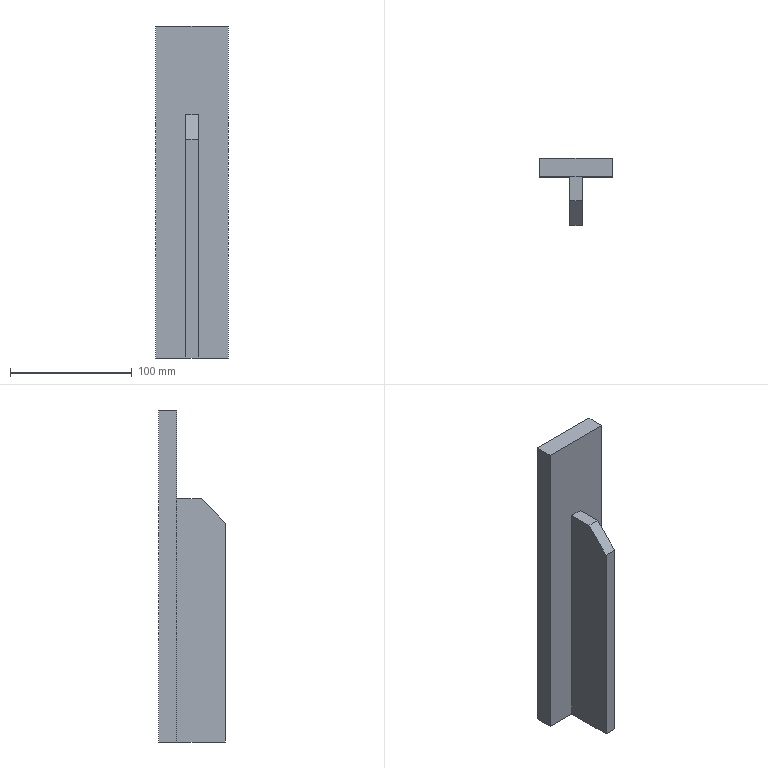Part | NX | features solid 2 | 1 solid | 11 faces | box 60 x 55 x 272.979 mm | volume 323681 mm3 | plane 11
STEP:
#1=CARTESIAN_POINT('',(5.,847.5,-310.));
#2=VERTEX_POINT('',#1);
#3=CARTESIAN_POINT('',(65.,847.5,-310.));
#4=VERTEX_POINT('',#3);
#5=CARTESIAN_POINT('',(9.058,847.5,-310.));
#6=DIRECTION('',(-1.,0.,0.));
#7=VECTOR('',#6,1000.);
#8=LINE('',#5,#7);
#9=EDGE_CURVE('',#2,#4,#8,.F.);
#10=ORIENTED_EDGE('',*,*,#9,.T.);
#11=CARTESIAN_POINT('',(65.,832.5,-310.));
#12=VERTEX_POINT('',#11);
#13=CARTESIAN_POINT('',(65.,840.,-310.));
#14=DIRECTION('',(0.,-1.,0.));
#15=VECTOR('',#14,1000.);
#16=LINE('',#13,#15);
#17=EDGE_CURVE('',#12,#4,#16,.F.);
#18=ORIENTED_EDGE('',*,*,#17,.F.);
#19=CARTESIAN_POINT('',(40.,832.5,-310.));
#20=VERTEX_POINT('',#19);
#21=CARTESIAN_POINT('',(9.058,832.5,-310.));
#22=DIRECTION('',(-1.,0.,0.));
#23=VECTOR('',#22,1000.);
#24=LINE('',#21,#23);
#25=EDGE_CURVE('',#20,#12,#24,.F.);
#26=ORIENTED_EDGE('',*,*,#25,.F.);
#27=CARTESIAN_POINT('',(40.,792.5,-310.));
#28=VERTEX_POINT('',#27);
#29=CARTESIAN_POINT('',(40.,832.5,-310.));
#30=DIRECTION('',(0.,-1.,0.));
#31=VECTOR('',#30,1000.);
#32=LINE('',#29,#31);
#33=EDGE_CURVE('',#20,#28,#32,.T.);
#34=ORIENTED_EDGE('',*,*,#33,.T.);
#35=CARTESIAN_POINT('',(30.,792.5,-310.));
#36=VERTEX_POINT('',#35);
#37=CARTESIAN_POINT('',(35.,792.5,-310.));
#38=DIRECTION('',(1.,0.,0.));
#39=VECTOR('',#38,1000.);
#40=LINE('',#37,#39);
#41=EDGE_CURVE('',#36,#28,#40,.T.);
#42=ORIENTED_EDGE('',*,*,#41,.F.);
#43=CARTESIAN_POINT('',(30.,832.5,-310.));
#44=VERTEX_POINT('',#43);
#45=CARTESIAN_POINT('',(30.,832.5,-310.));
#46=DIRECTION('',(0.,-1.,0.));
#47=VECTOR('',#46,1000.);
#48=LINE('',#45,#47);
#49=EDGE_CURVE('',#44,#36,#48,.T.);
#50=ORIENTED_EDGE('',*,*,#49,.F.);
#51=CARTESIAN_POINT('',(5.,832.5,-310.));
#52=VERTEX_POINT('',#51);
#53=CARTESIAN_POINT('',(9.058,832.5,-310.));
#54=DIRECTION('',(-1.,0.,0.));
#55=VECTOR('',#54,1000.);
#56=LINE('',#53,#55);
#57=EDGE_CURVE('',#52,#44,#56,.F.);
#58=ORIENTED_EDGE('',*,*,#57,.F.);
#59=CARTESIAN_POINT('',(5.,840.,-310.));
#60=DIRECTION('',(0.,-1.,0.));
#61=VECTOR('',#60,1000.);
#62=LINE('',#59,#61);
#63=EDGE_CURVE('',#52,#2,#62,.F.);
#64=ORIENTED_EDGE('',*,*,#63,.T.);
#65=EDGE_LOOP('',(#10,#18,#26,#34,#42,#50,#58,#64));
#66=FACE_BOUND('',#65,.T.);
#67=CARTESIAN_POINT('',(5.,847.5,-310.));
#68=DIRECTION('',(0.,0.,-1.));
#69=DIRECTION('',(-1.,0.,0.));
#70=AXIS2_PLACEMENT_3D('',#67,#68,#69);
#71=PLANE('',#70);
#72=ADVANCED_FACE('',(#66),#71,.T.);
#73=CARTESIAN_POINT('',(30.,812.5,-110.));
#74=VERTEX_POINT('',#73);
#75=CARTESIAN_POINT('',(30.,792.5,-130.));
#76=VERTEX_POINT('',#75);
#77=CARTESIAN_POINT('',(30.,792.5,-130.));
#78=DIRECTION('',(0.,-0.7071,-0.7071));
#79=VECTOR('',#78,1000.);
#80=LINE('',#77,#79);
#81=EDGE_CURVE('',#74,#76,#80,.T.);
#82=ORIENTED_EDGE('',*,*,#81,.T.);
#83=CARTESIAN_POINT('',(40.,792.5,-130.));
#84=VERTEX_POINT('',#83);
#85=CARTESIAN_POINT('',(35.,792.5,-130.));
#86=DIRECTION('',(1.,0.,0.));
#87=VECTOR('',#86,1000.);
#88=LINE('',#85,#87);
#89=EDGE_CURVE('',#76,#84,#88,.T.);
#90=ORIENTED_EDGE('',*,*,#89,.T.);
#91=CARTESIAN_POINT('',(40.,812.5,-110.));
#92=VERTEX_POINT('',#91);
#93=CARTESIAN_POINT('',(40.,722.5,-200.));
#94=DIRECTION('',(0.,0.7071,0.7071));
#95=VECTOR('',#94,1000.);
#96=LINE('',#93,#95);
#97=EDGE_CURVE('',#84,#92,#96,.T.);
#98=ORIENTED_EDGE('',*,*,#97,.T.);
#99=CARTESIAN_POINT('',(35.,812.5,-110.));
#100=DIRECTION('',(1.,0.,0.));
#101=VECTOR('',#100,1000.);
#102=LINE('',#99,#101);
#103=EDGE_CURVE('',#92,#74,#102,.F.);
#104=ORIENTED_EDGE('',*,*,#103,.T.);
#105=EDGE_LOOP('',(#82,#90,#98,#104));
#106=FACE_BOUND('',#105,.T.);
#107=CARTESIAN_POINT('',(35.,792.5,-130.));
#108=DIRECTION('',(0.,-0.7071,0.7071));
#109=DIRECTION('',(0.,0.7071,0.7071));
#110=AXIS2_PLACEMENT_3D('',#107,#108,#109);
#111=PLANE('',#110);
#112=ADVANCED_FACE('',(#106),#111,.T.);
#113=CARTESIAN_POINT('',(40.,832.5,-110.));
#114=VERTEX_POINT('',#113);
#115=CARTESIAN_POINT('',(40.,832.5,-110.));
#116=DIRECTION('',(0.,-1.,0.));
#117=VECTOR('',#116,1000.);
#118=LINE('',#115,#117);
#119=EDGE_CURVE('',#114,#92,#118,.T.);
#120=ORIENTED_EDGE('',*,*,#119,.F.);
#121=CARTESIAN_POINT('',(30.,832.5,-110.));
#122=VERTEX_POINT('',#121);
#123=CARTESIAN_POINT('',(35.,832.5,-110.));
#124=DIRECTION('',(1.,0.,0.));
#125=VECTOR('',#124,1000.);
#126=LINE('',#123,#125);
#127=EDGE_CURVE('',#122,#114,#126,.T.);
#128=ORIENTED_EDGE('',*,*,#127,.F.);
#129=CARTESIAN_POINT('',(30.,832.5,-110.));
#130=DIRECTION('',(0.,-1.,0.));
#131=VECTOR('',#130,1000.);
#132=LINE('',#129,#131);
#133=EDGE_CURVE('',#122,#74,#132,.T.);
#134=ORIENTED_EDGE('',*,*,#133,.T.);
#135=ORIENTED_EDGE('',*,*,#103,.F.);
#136=EDGE_LOOP('',(#120,#128,#134,#135));
#137=FACE_BOUND('',#136,.T.);
#138=CARTESIAN_POINT('',(35.,832.5,-110.));
#139=DIRECTION('',(0.,0.,-1.));
#140=DIRECTION('',(0.,-1.,0.));
#141=AXIS2_PLACEMENT_3D('',#138,#139,#140);
#142=PLANE('',#141);
#143=ADVANCED_FACE('',(#137),#142,.F.);
#144=CARTESIAN_POINT('',(65.,832.5,-37.021));
#145=VERTEX_POINT('',#144);
#146=CARTESIAN_POINT('',(5.,832.5,-37.021));
#147=VERTEX_POINT('',#146);
#148=CARTESIAN_POINT('',(9.058,832.5,-37.021));
#149=DIRECTION('',(-1.,0.,0.));
#150=VECTOR('',#149,1000.);
#151=LINE('',#148,#150);
#152=EDGE_CURVE('',#145,#147,#151,.T.);
#153=ORIENTED_EDGE('',*,*,#152,.T.);
#154=CARTESIAN_POINT('',(5.,832.5,-21.795));
#155=DIRECTION('',(0.,0.,-1.));
#156=VECTOR('',#155,1000.);
#157=LINE('',#154,#156);
#158=EDGE_CURVE('',#147,#52,#157,.T.);
#159=ORIENTED_EDGE('',*,*,#158,.T.);
#160=ORIENTED_EDGE('',*,*,#57,.T.);
#161=CARTESIAN_POINT('',(30.,832.5,-310.));
#162=DIRECTION('',(0.,0.,1.));
#163=VECTOR('',#162,1000.);
#164=LINE('',#161,#163);
#165=EDGE_CURVE('',#44,#122,#164,.T.);
#166=ORIENTED_EDGE('',*,*,#165,.T.);
#167=ORIENTED_EDGE('',*,*,#127,.T.);
#168=CARTESIAN_POINT('',(40.,832.5,-310.));
#169=DIRECTION('',(0.,0.,1.));
#170=VECTOR('',#169,1000.);
#171=LINE('',#168,#170);
#172=EDGE_CURVE('',#20,#114,#171,.T.);
#173=ORIENTED_EDGE('',*,*,#172,.F.);
#174=ORIENTED_EDGE('',*,*,#25,.T.);
#175=CARTESIAN_POINT('',(65.,832.5,-51.379));
#176=DIRECTION('',(0.,0.,1.));
#177=VECTOR('',#176,1000.);
#178=LINE('',#175,#177);
#179=EDGE_CURVE('',#145,#12,#178,.F.);
#180=ORIENTED_EDGE('',*,*,#179,.F.);
#181=EDGE_LOOP('',(#153,#159,#160,#166,#167,#173,#174,#180));
#182=FACE_BOUND('',#181,.T.);
#183=CARTESIAN_POINT('',(9.058,832.5,-21.795));
#184=DIRECTION('',(0.,-1.,0.));
#185=DIRECTION('',(-1.,0.,0.));
#186=AXIS2_PLACEMENT_3D('',#183,#184,#185);
#187=PLANE('',#186);
#188=ADVANCED_FACE('',(#182),#187,.T.);
#189=CARTESIAN_POINT('',(40.,792.5,-310.));
#190=DIRECTION('',(0.,0.,1.));
#191=VECTOR('',#190,1000.);
#192=LINE('',#189,#191);
#193=EDGE_CURVE('',#28,#84,#192,.T.);
#194=ORIENTED_EDGE('',*,*,#193,.F.);
#195=ORIENTED_EDGE('',*,*,#33,.F.);
#196=ORIENTED_EDGE('',*,*,#172,.T.);
#197=ORIENTED_EDGE('',*,*,#119,.T.);
#198=ORIENTED_EDGE('',*,*,#97,.F.);
#199=EDGE_LOOP('',(#194,#195,#196,#197,#198));
#200=FACE_BOUND('',#199,.T.);
#201=CARTESIAN_POINT('',(40.,832.5,-310.));
#202=DIRECTION('',(1.,0.,0.));
#203=DIRECTION('',(0.,-1.,0.));
#204=AXIS2_PLACEMENT_3D('',#201,#202,#203);
#205=PLANE('',#204);
#206=ADVANCED_FACE('',(#200),#205,.T.);
#207=CARTESIAN_POINT('',(30.,792.5,-310.));
#208=DIRECTION('',(0.,0.,1.));
#209=VECTOR('',#208,1000.);
#210=LINE('',#207,#209);
#211=EDGE_CURVE('',#36,#76,#210,.T.);
#212=ORIENTED_EDGE('',*,*,#211,.F.);
#213=ORIENTED_EDGE('',*,*,#41,.T.);
#214=ORIENTED_EDGE('',*,*,#193,.T.);
#215=ORIENTED_EDGE('',*,*,#89,.F.);
#216=EDGE_LOOP('',(#212,#213,#214,#215));
#217=FACE_BOUND('',#216,.T.);
#218=CARTESIAN_POINT('',(35.,792.5,-310.));
#219=DIRECTION('',(0.,-1.,0.));
#220=DIRECTION('',(0.,0.,1.));
#221=AXIS2_PLACEMENT_3D('',#218,#219,#220);
#222=PLANE('',#221);
#223=ADVANCED_FACE('',(#217),#222,.T.);
#224=ORIENTED_EDGE('',*,*,#133,.F.);
#225=ORIENTED_EDGE('',*,*,#165,.F.);
#226=ORIENTED_EDGE('',*,*,#49,.T.);
#227=ORIENTED_EDGE('',*,*,#211,.T.);
#228=ORIENTED_EDGE('',*,*,#81,.F.);
#229=EDGE_LOOP('',(#224,#225,#226,#227,#228));
#230=FACE_BOUND('',#229,.T.);
#231=CARTESIAN_POINT('',(30.,832.5,-310.));
#232=DIRECTION('',(1.,0.,0.));
#233=DIRECTION('',(0.,-1.,0.));
#234=AXIS2_PLACEMENT_3D('',#231,#232,#233);
#235=PLANE('',#234);
#236=ADVANCED_FACE('',(#230),#235,.F.);
#237=CARTESIAN_POINT('',(5.,847.5,-37.021));
#238=VERTEX_POINT('',#237);
#239=CARTESIAN_POINT('',(5.,847.5,-21.795));
#240=DIRECTION('',(0.,0.,-1.));
#241=VECTOR('',#240,1000.);
#242=LINE('',#239,#241);
#243=EDGE_CURVE('',#238,#2,#242,.T.);
#244=ORIENTED_EDGE('',*,*,#243,.T.);
#245=ORIENTED_EDGE('',*,*,#63,.F.);
#246=ORIENTED_EDGE('',*,*,#158,.F.);
#247=CARTESIAN_POINT('',(5.,840.,-37.021));
#248=DIRECTION('',(0.,-1.,0.));
#249=VECTOR('',#248,1000.);
#250=LINE('',#247,#249);
#251=EDGE_CURVE('',#238,#147,#250,.T.);
#252=ORIENTED_EDGE('',*,*,#251,.F.);
#253=EDGE_LOOP('',(#244,#245,#246,#252));
#254=FACE_BOUND('',#253,.T.);
#255=CARTESIAN_POINT('',(5.,840.,-21.795));
#256=DIRECTION('',(1.,0.,0.));
#257=DIRECTION('',(0.,0.,-1.));
#258=AXIS2_PLACEMENT_3D('',#255,#256,#257);
#259=PLANE('',#258);
#260=ADVANCED_FACE('',(#254),#259,.F.);
#261=CARTESIAN_POINT('',(65.,847.5,-37.021));
#262=VERTEX_POINT('',#261);
#263=CARTESIAN_POINT('',(65.,847.5,-51.379));
#264=DIRECTION('',(0.,0.,1.));
#265=VECTOR('',#264,1000.);
#266=LINE('',#263,#265);
#267=EDGE_CURVE('',#262,#4,#266,.F.);
#268=ORIENTED_EDGE('',*,*,#267,.T.);
#269=ORIENTED_EDGE('',*,*,#9,.F.);
#270=ORIENTED_EDGE('',*,*,#243,.F.);
#271=CARTESIAN_POINT('',(9.058,847.5,-37.021));
#272=DIRECTION('',(-1.,0.,0.));
#273=VECTOR('',#272,1000.);
#274=LINE('',#271,#273);
#275=EDGE_CURVE('',#262,#238,#274,.T.);
#276=ORIENTED_EDGE('',*,*,#275,.F.);
#277=EDGE_LOOP('',(#268,#269,#270,#276));
#278=FACE_BOUND('',#277,.T.);
#279=CARTESIAN_POINT('',(9.058,847.5,-21.795));
#280=DIRECTION('',(0.,-1.,0.));
#281=DIRECTION('',(-1.,0.,0.));
#282=AXIS2_PLACEMENT_3D('',#279,#280,#281);
#283=PLANE('',#282);
#284=ADVANCED_FACE('',(#278),#283,.F.);
#285=ORIENTED_EDGE('',*,*,#179,.T.);
#286=ORIENTED_EDGE('',*,*,#17,.T.);
#287=ORIENTED_EDGE('',*,*,#267,.F.);
#288=CARTESIAN_POINT('',(65.,840.,-37.021));
#289=DIRECTION('',(0.,-1.,0.));
#290=VECTOR('',#289,1000.);
#291=LINE('',#288,#290);
#292=EDGE_CURVE('',#145,#262,#291,.F.);
#293=ORIENTED_EDGE('',*,*,#292,.F.);
#294=EDGE_LOOP('',(#285,#286,#287,#293));
#295=FACE_BOUND('',#294,.T.);
#296=CARTESIAN_POINT('',(65.,840.,-51.379));
#297=DIRECTION('',(1.,0.,0.));
#298=DIRECTION('',(0.,0.,-1.));
#299=AXIS2_PLACEMENT_3D('',#296,#297,#298);
#300=PLANE('',#299);
#301=ADVANCED_FACE('',(#295),#300,.T.);
#302=ORIENTED_EDGE('',*,*,#152,.F.);
#303=ORIENTED_EDGE('',*,*,#292,.T.);
#304=ORIENTED_EDGE('',*,*,#275,.T.);
#305=ORIENTED_EDGE('',*,*,#251,.T.);
#306=EDGE_LOOP('',(#302,#303,#304,#305));
#307=FACE_BOUND('',#306,.T.);
#308=CARTESIAN_POINT('',(54.128,890.,-37.021));
#309=DIRECTION('',(0.,0.,-1.));
#310=DIRECTION('',(-1.,0.,0.));
#311=AXIS2_PLACEMENT_3D('',#308,#309,#310);
#312=PLANE('',#311);
#313=ADVANCED_FACE('',(#307),#312,.F.);
#314=CLOSED_SHELL('',(#72,#112,#143,#188,#206,#223,#236,#260,#284,#301,#313));
#315=MANIFOLD_SOLID_BREP('',#314);
#316=(LENGTH_UNIT()NAMED_UNIT(*)SI_UNIT(.MILLI.,.METRE.));
#317=UNCERTAINTY_MEASURE_WITH_UNIT(LENGTH_MEASURE(0.00001),#316,'','');
#318=(NAMED_UNIT(*)PLANE_ANGLE_UNIT()SI_UNIT($,.RADIAN.));
#319=(NAMED_UNIT(*)SI_UNIT($,.STERADIAN.)SOLID_ANGLE_UNIT());
#320=(GEOMETRIC_REPRESENTATION_CONTEXT(3)GLOBAL_UNCERTAINTY_ASSIGNED_CONTEXT((#317))GLOBAL_UNIT_ASSIGNED_CONTEXT((#316,#318,#319))REPRESENTATION_CONTEXT('',''));
#321=ADVANCED_BREP_SHAPE_REPRESENTATION('',(#315),#320);